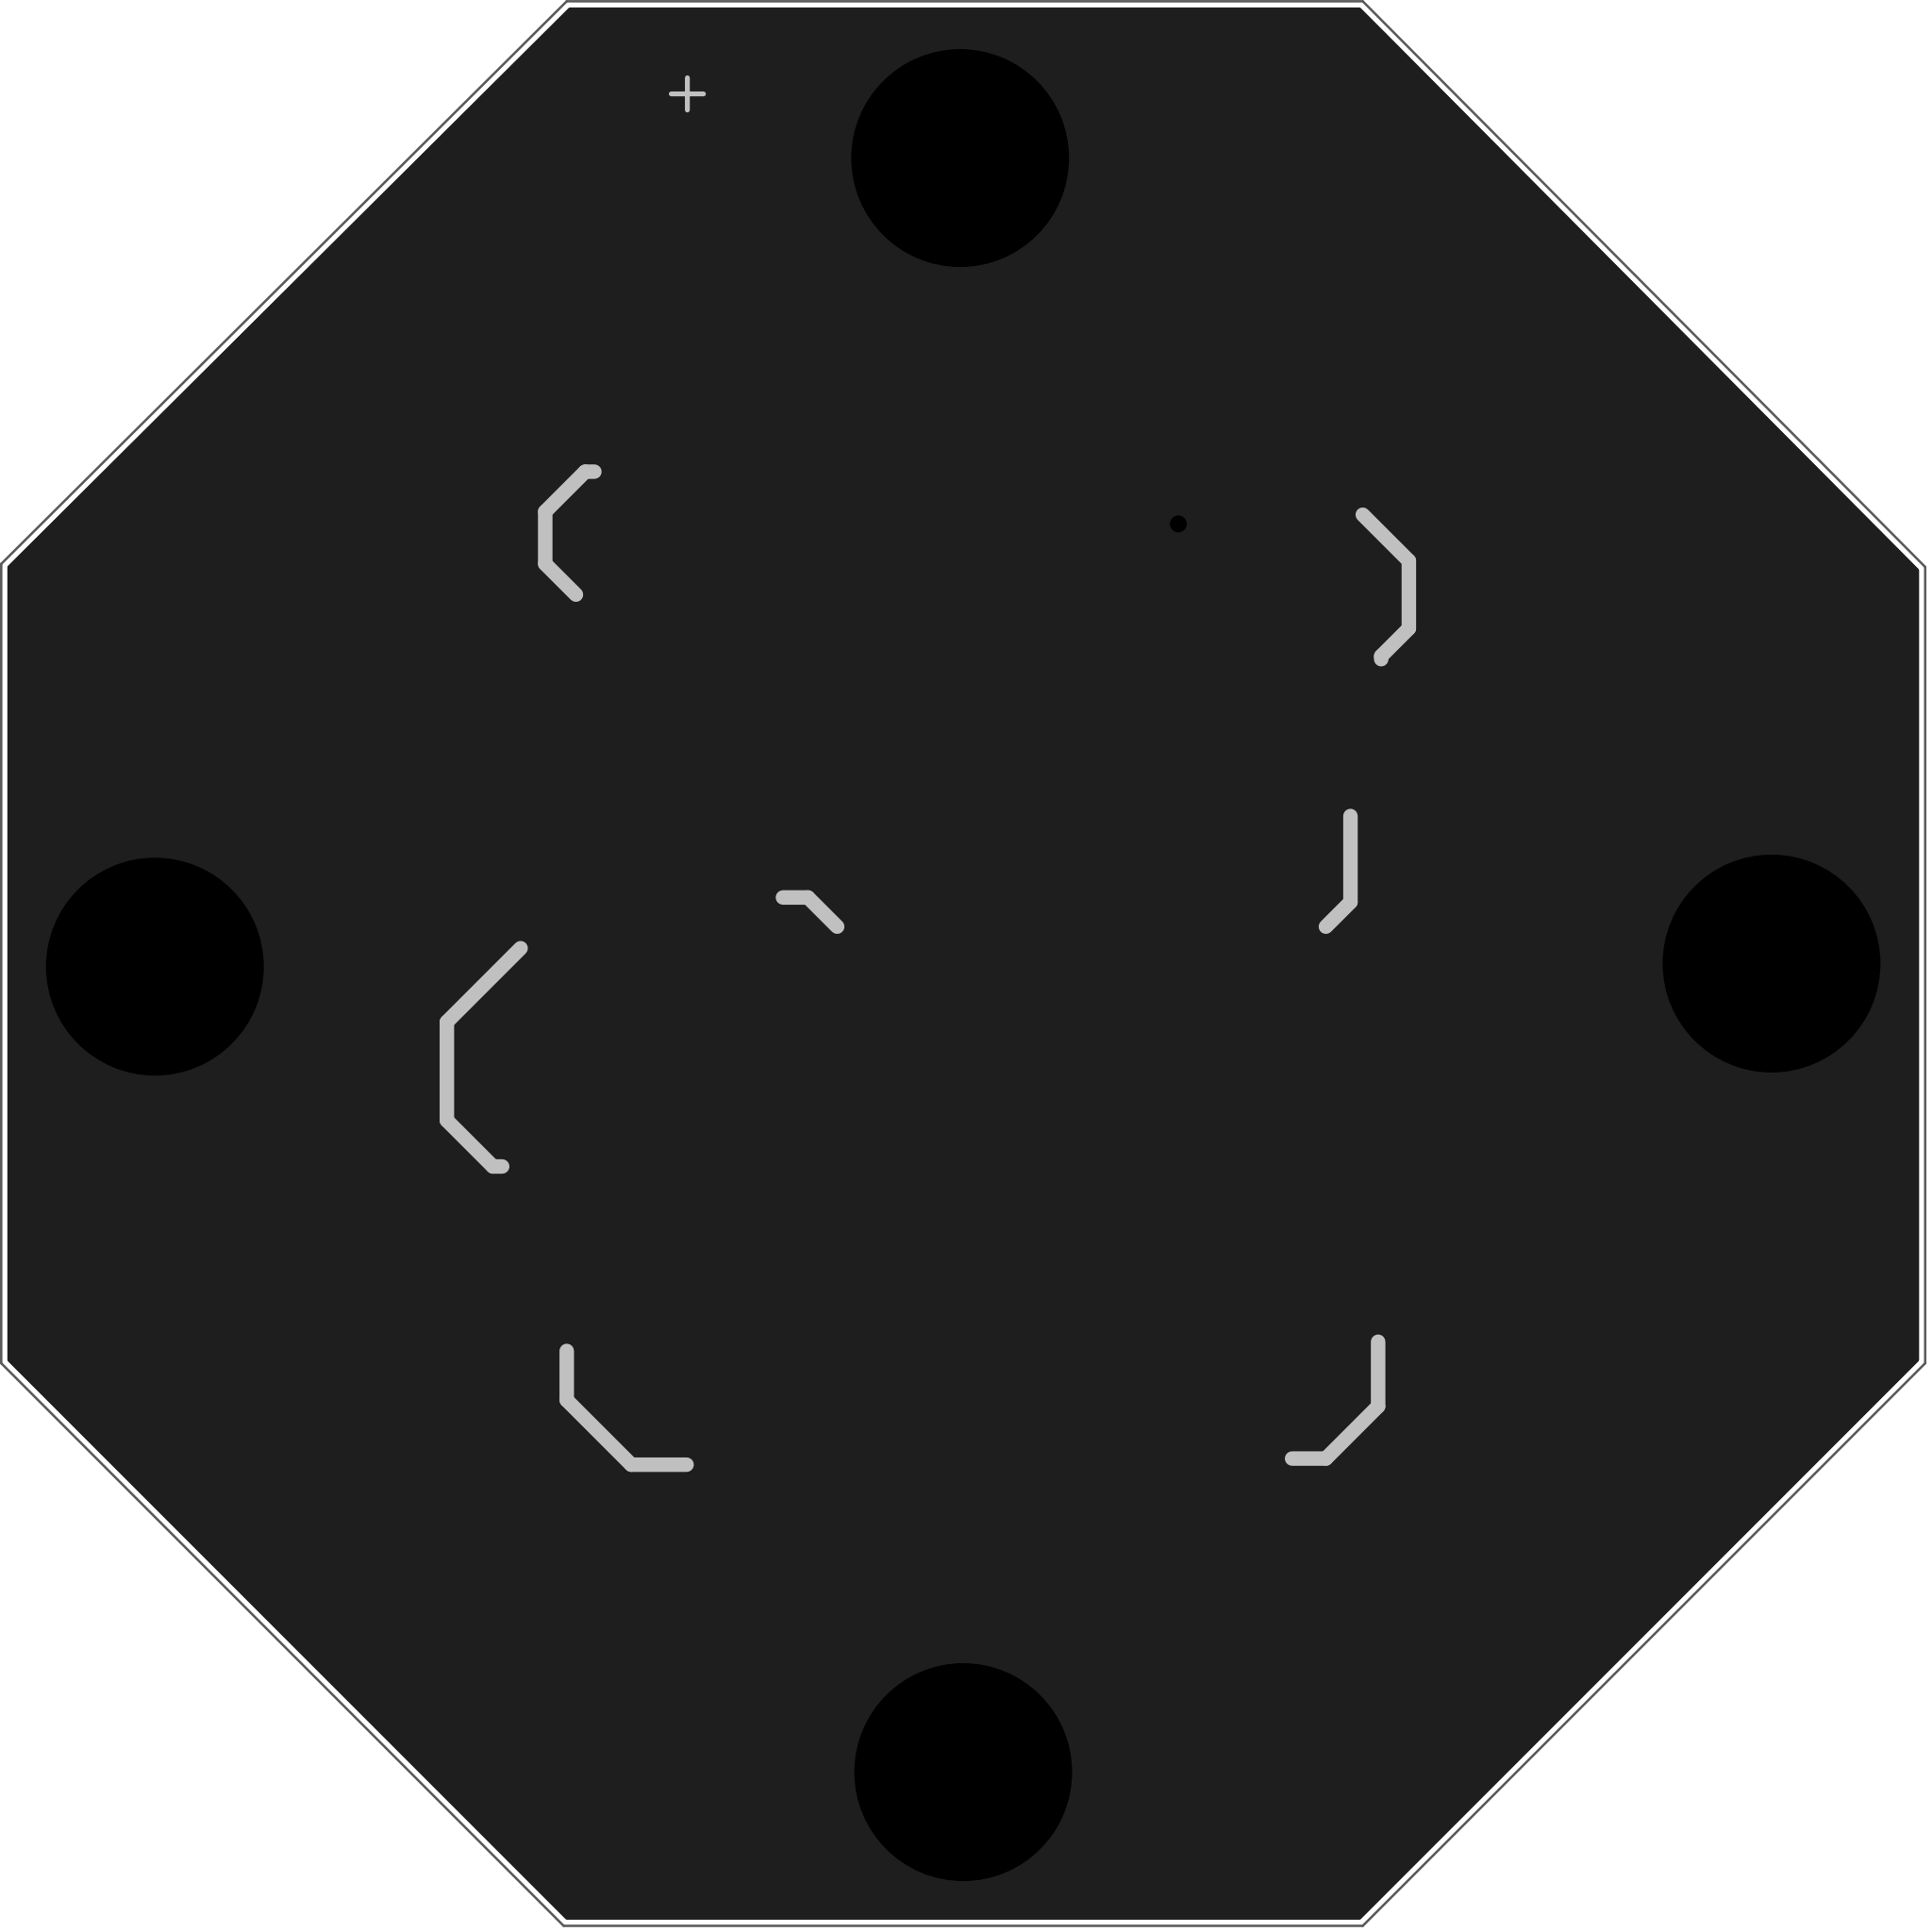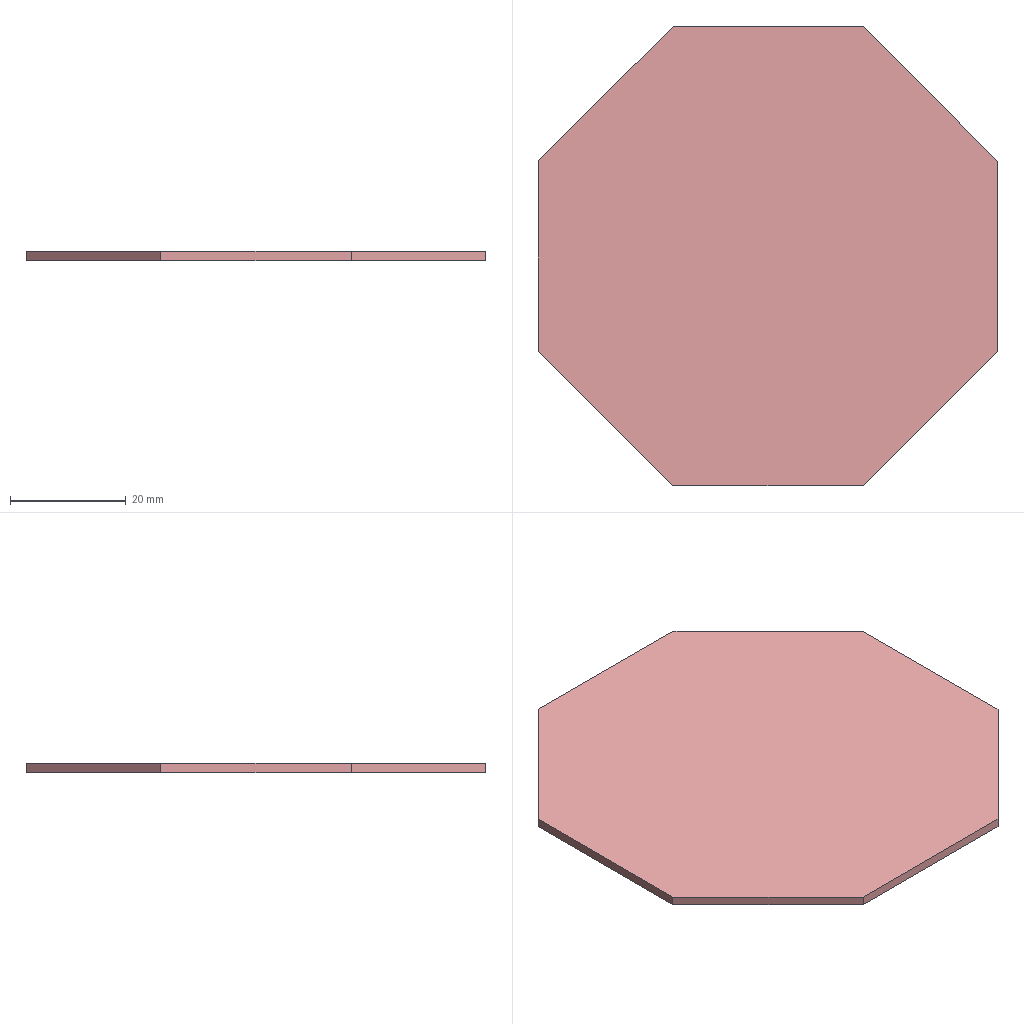Circuit board layout | Altium Designer | box 79.5 x 79.5 x 1.6 mm
Layer stack:
# Altium Designer layer stack of  (unit mm; dielectric type: 0 none, 1 core, 2 prepreg, 3 surface material)
index,name,kind,layer,copper_thickness_mm,dielectric_type,dielectric_thickness_mm,dielectric_material,dielectric_constant
0,Top Paste Mask Layer,other,,,,,,
1,Top Silkscreen Layer,other,,,,,,
2,Top Solder Mask Layer,dielectric,,,3,0.01,,3.3
3,Top Layer,copper,Top Layer,0.035,,,,
4,Dielectric1,dielectric,,,3,1.51,FR4,4.5
5,Bottom Layer,copper,Bottom Layer,0.035,,,,
6,Bottom Solder Mask Layer,dielectric,,,3,0.01,,3.3
7,Bottom Silkscreen Layer,other,,,,,,
8,Bottom Paste Mask Layer,other,,,,,,
# drill layer pairs: low layer,high layer
drill_pair,Top Layer,Bottom Layer
Part placement:
Designator,Comment,Layer,Footprint,Center-X(mm),Center-Y(mm),Rotation
LED1,,BottomLayer,LED_0603,142.408,142.571,225
LED2,,BottomLayer,LED_0603,142.644,92.933,135
LED3,,BottomLayer,LED_0603,88.986,93.742,45
LED4,,BottomLayer,LED_0603,89.135,142.817,315
R1,3.3k,BottomLayer,R0603,141.097,143.81,225
R2,3.3k,BottomLayer,R0603,141.725,91.959,135
R3,3.3k,BottomLayer,R0603,90.17,92.629,45
R4,3.3k,BottomLayer,R0603,90.551,144.064,315
Pad and via stacks:
# Altium Designer via and pad stacks of  (unit mm). Each distinct definition once, with the count of objects using it.
# via: kind,start_layer,end_layer,hole_mm,diameter_mm,mode(0 simple;1 top-mid-bottom;2 full stack),diameter_per_layer,count,example_net
# pad: kind,layer,hole_mm,hole_type(0 round;1 square;2 slot),plating,top_size,top_shape(1 round;2 rect;3 octagon;9 rounded rect),mid_size,bottom_size,mode,footprint,size_per_layer,count,example
pad,Bottom Layer,0,0,plated,0.8001x0.8001,2,0.8001x0.8001,0.8001x0.8001,0,LED_0603,,8,LED1.1
pad,Bottom Layer,0,0,plated,0.8065x0.864,2,0.8065x0.864,0.8065x0.864,0,R0603,,8,R1.2
via,Top Layer,Bottom Layer,6,9,0,,4,+5V
via,Top Layer,Bottom Layer,0.3988,0.7,0,,1,+5V
Copper pours:
name,layer,net,type(0 solid;1 hatched;2 none)
Top Layer-+5V,Top Layer,+5V,0
Bottom Layer-GND,Bottom Layer,GND,0